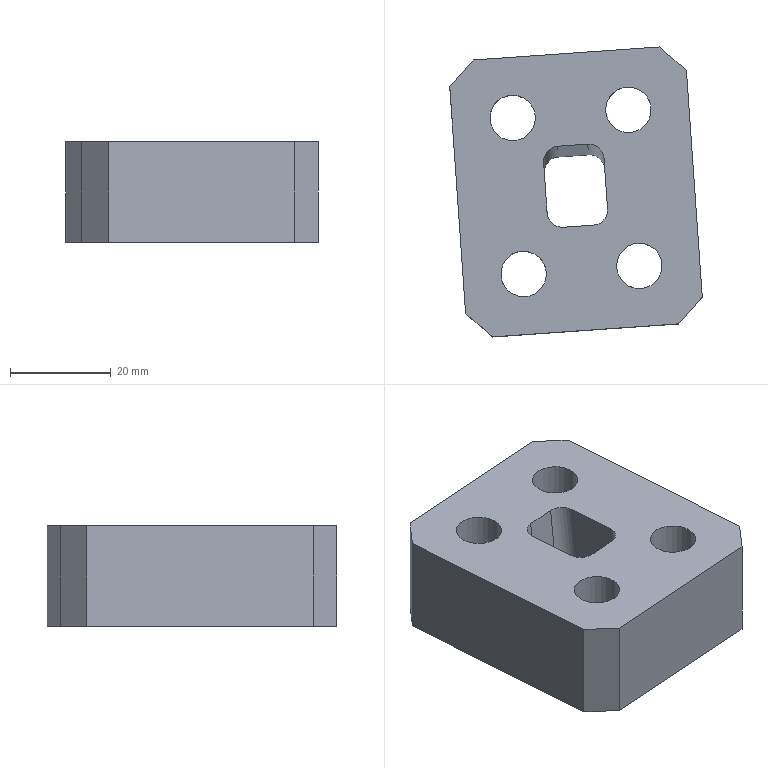Part | STEP file | 车灯-后视镜_id158_x_t | 1 solid | 30 faces | box 50.025 x 57.447 x 20 mm | volume 38834 mm3 | plane 18 | cylinder 12 | commonest cylinder face diameters 6 x4 9 x4 14 x4
STEP:
#1=CARTESIAN_POINT('',(-10.346,-54.305,-160.5));
#2=VERTEX_POINT('',#1);
#3=CARTESIAN_POINT('',(-10.346,-61.305,-160.5));
#4=DIRECTION('',(0.,0.,1.));
#5=DIRECTION('',(0.,1.,0.));
#6=AXIS2_PLACEMENT_3D('',#3,#4,#5);
#7=CIRCLE('',#6,7.);
#8=EDGE_CURVE('',#2,#2,#7,.T.);
#9=ORIENTED_EDGE('',*,*,#8,.T.);
#10=EDGE_LOOP('',(#9));
#11=FACE_BOUND('',#10,.T.);
#12=CARTESIAN_POINT('',(-8.184,-85.229,-160.5));
#13=VERTEX_POINT('',#12);
#14=CARTESIAN_POINT('',(-8.184,-92.229,-160.5));
#15=DIRECTION('',(0.,0.,-1.));
#16=DIRECTION('',(0.,1.,0.));
#17=AXIS2_PLACEMENT_3D('',#14,#15,#16);
#18=CIRCLE('',#17,7.);
#19=EDGE_CURVE('',#13,#13,#18,.T.);
#20=ORIENTED_EDGE('',*,*,#19,.F.);
#21=EDGE_LOOP('',(#20));
#22=FACE_BOUND('',#21,.T.);
#23=CARTESIAN_POINT('',(12.598,-52.7,-160.5));
#24=VERTEX_POINT('',#23);
#25=CARTESIAN_POINT('',(12.598,-59.7,-160.5));
#26=DIRECTION('',(0.,0.,-1.));
#27=DIRECTION('',(0.,1.,0.));
#28=AXIS2_PLACEMENT_3D('',#25,#26,#27);
#29=CIRCLE('',#28,7.);
#30=EDGE_CURVE('',#24,#24,#29,.T.);
#31=ORIENTED_EDGE('',*,*,#30,.F.);
#32=EDGE_LOOP('',(#31));
#33=FACE_BOUND('',#32,.T.);
#34=CARTESIAN_POINT('',(14.76,-83.625,-160.5));
#35=VERTEX_POINT('',#34);
#36=CARTESIAN_POINT('',(14.76,-90.625,-160.5));
#37=DIRECTION('',(0.,0.,1.));
#38=DIRECTION('',(0.,1.,0.));
#39=AXIS2_PLACEMENT_3D('',#36,#37,#38);
#40=CIRCLE('',#39,7.);
#41=EDGE_CURVE('',#35,#35,#40,.T.);
#42=ORIENTED_EDGE('',*,*,#41,.T.);
#43=EDGE_LOOP('',(#42));
#44=FACE_BOUND('',#43,.T.);
#45=CARTESIAN_POINT('',(-18.166,-49.822,-160.5));
#46=VERTEX_POINT('',#45);
#47=CARTESIAN_POINT('',(18.744,-47.241,-160.5));
#48=VERTEX_POINT('',#47);
#49=CARTESIAN_POINT('',(0.8645,-48.491,-160.5));
#50=DIRECTION('',(0.9976,0.06976,0.));
#51=VECTOR('',#50,1.);
#52=LINE('',#49,#51);
#53=EDGE_CURVE('',#46,#48,#52,.T.);
#54=ORIENTED_EDGE('',*,*,#53,.T.);
#55=CARTESIAN_POINT('',(24.08,-51.88,-160.5));
#56=VERTEX_POINT('',#55);
#57=CARTESIAN_POINT('',(18.744,-47.241,-160.5));
#58=DIRECTION('',(-0.7547,0.6561,0.));
#59=VECTOR('',#58,1.);
#60=LINE('',#57,#59);
#61=EDGE_CURVE('',#56,#48,#60,.T.);
#62=ORIENTED_EDGE('',*,*,#61,.F.);
#63=CARTESIAN_POINT('',(27.219,-96.771,-160.5));
#64=VERTEX_POINT('',#63);
#65=CARTESIAN_POINT('',(26.697,-89.301,-160.5));
#66=DIRECTION('',(0.06976,-0.9976,0.));
#67=VECTOR('',#66,1.);
#68=LINE('',#65,#67);
#69=EDGE_CURVE('',#56,#64,#68,.T.);
#70=ORIENTED_EDGE('',*,*,#69,.T.);
#71=CARTESIAN_POINT('',(22.58,-102.107,-160.5));
#72=VERTEX_POINT('',#71);
#73=CARTESIAN_POINT('',(22.58,-102.107,-160.5));
#74=DIRECTION('',(0.6561,0.7547,0.));
#75=VECTOR('',#74,1.);
#76=LINE('',#73,#75);
#77=EDGE_CURVE('',#72,#64,#76,.T.);
#78=ORIENTED_EDGE('',*,*,#77,.F.);
#79=CARTESIAN_POINT('',(-14.33,-104.688,-160.5));
#80=VERTEX_POINT('',#79);
#81=CARTESIAN_POINT('',(4.701,-103.357,-160.5));
#82=DIRECTION('',(-0.9976,-0.06976,0.));
#83=VECTOR('',#82,1.);
#84=LINE('',#81,#83);
#85=EDGE_CURVE('',#72,#80,#84,.T.);
#86=ORIENTED_EDGE('',*,*,#85,.T.);
#87=CARTESIAN_POINT('',(-19.666,-100.049,-160.5));
#88=VERTEX_POINT('',#87);
#89=CARTESIAN_POINT('',(-14.33,-104.688,-160.5));
#90=DIRECTION('',(0.7547,-0.6561,0.));
#91=VECTOR('',#90,1.);
#92=LINE('',#89,#91);
#93=EDGE_CURVE('',#88,#80,#92,.T.);
#94=ORIENTED_EDGE('',*,*,#93,.F.);
#95=CARTESIAN_POINT('',(-22.805,-55.159,-160.5));
#96=VERTEX_POINT('',#95);
#97=CARTESIAN_POINT('',(-20.188,-92.579,-160.5));
#98=DIRECTION('',(-0.06976,0.9976,0.));
#99=VECTOR('',#98,1.);
#100=LINE('',#97,#99);
#101=EDGE_CURVE('',#88,#96,#100,.T.);
#102=ORIENTED_EDGE('',*,*,#101,.T.);
#103=CARTESIAN_POINT('',(-22.805,-55.159,-160.5));
#104=DIRECTION('',(-0.6561,-0.7547,0.));
#105=VECTOR('',#104,1.);
#106=LINE('',#103,#105);
#107=EDGE_CURVE('',#46,#96,#106,.T.);
#108=ORIENTED_EDGE('',*,*,#107,.F.);
#109=EDGE_LOOP('',(#54,#62,#70,#78,#86,#94,#102,#108));
#110=FACE_BOUND('',#109,.T.);
#111=CARTESIAN_POINT('',(-4.069,-72.231,-160.5));
#112=VERTEX_POINT('',#111);
#113=CARTESIAN_POINT('',(-1.286,-69.013,-160.5));
#114=VERTEX_POINT('',#113);
#115=CARTESIAN_POINT('',(-1.076,-72.022,-160.5));
#116=DIRECTION('',(0.,0.,-1.));
#117=DIRECTION('',(-0.06976,0.9976,0.));
#118=AXIS2_PLACEMENT_3D('',#115,#116,#117);
#119=ELLIPSE('',#118,3.017,3.);
#120=EDGE_CURVE('',#112,#114,#119,.T.);
#121=ORIENTED_EDGE('',*,*,#120,.F.);
#122=CARTESIAN_POINT('',(-3.367,-82.262,-160.5));
#123=VERTEX_POINT('',#122);
#124=CARTESIAN_POINT('',(-2.731,-91.358,-160.5));
#125=DIRECTION('',(0.06976,-0.9976,0.));
#126=VECTOR('',#125,1.);
#127=LINE('',#124,#126);
#128=EDGE_CURVE('',#112,#123,#127,.T.);
#129=ORIENTED_EDGE('',*,*,#128,.T.);
#130=CARTESIAN_POINT('',(-0.1641,-85.062,-160.5));
#131=VERTEX_POINT('',#130);
#132=CARTESIAN_POINT('',(-0.3745,-82.053,-160.5));
#133=DIRECTION('',(0.,0.,-1.));
#134=DIRECTION('',(0.06976,-0.9976,0.));
#135=AXIS2_PLACEMENT_3D('',#132,#133,#134);
#136=ELLIPSE('',#135,3.017,3.);
#137=EDGE_CURVE('',#131,#123,#136,.T.);
#138=ORIENTED_EDGE('',*,*,#137,.F.);
#139=CARTESIAN_POINT('',(5.821,-84.643,-160.5));
#140=VERTEX_POINT('',#139);
#141=CARTESIAN_POINT('',(3.404,-84.812,-160.5));
#142=DIRECTION('',(-0.9976,-0.06976,0.));
#143=VECTOR('',#142,1.);
#144=LINE('',#141,#143);
#145=EDGE_CURVE('',#140,#131,#144,.T.);
#146=ORIENTED_EDGE('',*,*,#145,.F.);
#147=CARTESIAN_POINT('',(8.604,-81.425,-160.5));
#148=VERTEX_POINT('',#147);
#149=CARTESIAN_POINT('',(5.611,-81.634,-160.5));
#150=DIRECTION('',(0.,0.,-1.));
#151=DIRECTION('',(-0.06976,0.9976,0.));
#152=AXIS2_PLACEMENT_3D('',#149,#150,#151);
#153=ELLIPSE('',#152,3.017,3.);
#154=EDGE_CURVE('',#148,#140,#153,.T.);
#155=ORIENTED_EDGE('',*,*,#154,.F.);
#156=CARTESIAN_POINT('',(7.902,-71.394,-160.5));
#157=VERTEX_POINT('',#156);
#158=CARTESIAN_POINT('',(9.24,-90.521,-160.5));
#159=DIRECTION('',(0.06976,-0.9976,0.));
#160=VECTOR('',#159,1.);
#161=LINE('',#158,#160);
#162=EDGE_CURVE('',#157,#148,#161,.T.);
#163=ORIENTED_EDGE('',*,*,#162,.F.);
#164=CARTESIAN_POINT('',(4.699,-68.594,-160.5));
#165=VERTEX_POINT('',#164);
#166=CARTESIAN_POINT('',(4.909,-71.603,-160.5));
#167=DIRECTION('',(0.,0.,-1.));
#168=DIRECTION('',(0.06976,-0.9976,0.));
#169=AXIS2_PLACEMENT_3D('',#166,#167,#168);
#170=ELLIPSE('',#169,3.017,3.);
#171=EDGE_CURVE('',#165,#157,#170,.T.);
#172=ORIENTED_EDGE('',*,*,#171,.F.);
#173=CARTESIAN_POINT('',(2.282,-68.763,-160.5));
#174=DIRECTION('',(0.9976,0.06976,0.));
#175=VECTOR('',#174,1.);
#176=LINE('',#173,#175);
#177=EDGE_CURVE('',#114,#165,#176,.T.);
#178=ORIENTED_EDGE('',*,*,#177,.F.);
#179=EDGE_LOOP('',(#121,#129,#138,#146,#155,#163,#172,#178));
#180=FACE_BOUND('',#179,.T.);
#181=CARTESIAN_POINT('',(3.83,-90.9,-160.5));
#182=DIRECTION('',(0.,0.,-1.));
#183=DIRECTION('',(-0.06976,0.9976,0.));
#184=AXIS2_PLACEMENT_3D('',#181,#182,#183);
#185=PLANE('',#184);
#186=ADVANCED_FACE('',(#11,#22,#33,#44,#110,#180),#185,.T.);
#187=CARTESIAN_POINT('',(-10.346,-65.805,-140.5));
#188=VERTEX_POINT('',#187);
#189=CARTESIAN_POINT('',(-10.346,-61.305,-140.5));
#190=DIRECTION('',(0.,0.,-1.));
#191=DIRECTION('',(0.,-1.,0.));
#192=AXIS2_PLACEMENT_3D('',#189,#190,#191);
#193=CIRCLE('',#192,4.5);
#194=EDGE_CURVE('',#188,#188,#193,.T.);
#195=ORIENTED_EDGE('',*,*,#194,.T.);
#196=EDGE_LOOP('',(#195));
#197=FACE_BOUND('',#196,.T.);
#198=CARTESIAN_POINT('',(-8.184,-96.729,-140.5));
#199=VERTEX_POINT('',#198);
#200=CARTESIAN_POINT('',(-8.184,-92.229,-140.5));
#201=DIRECTION('',(0.,0.,1.));
#202=DIRECTION('',(0.,-1.,0.));
#203=AXIS2_PLACEMENT_3D('',#200,#201,#202);
#204=CIRCLE('',#203,4.5);
#205=EDGE_CURVE('',#199,#199,#204,.T.);
#206=ORIENTED_EDGE('',*,*,#205,.F.);
#207=EDGE_LOOP('',(#206));
#208=FACE_BOUND('',#207,.T.);
#209=CARTESIAN_POINT('',(12.598,-64.2,-140.5));
#210=VERTEX_POINT('',#209);
#211=CARTESIAN_POINT('',(12.598,-59.7,-140.5));
#212=DIRECTION('',(0.,0.,1.));
#213=DIRECTION('',(0.,-1.,0.));
#214=AXIS2_PLACEMENT_3D('',#211,#212,#213);
#215=CIRCLE('',#214,4.5);
#216=EDGE_CURVE('',#210,#210,#215,.T.);
#217=ORIENTED_EDGE('',*,*,#216,.F.);
#218=EDGE_LOOP('',(#217));
#219=FACE_BOUND('',#218,.T.);
#220=CARTESIAN_POINT('',(14.76,-95.125,-140.5));
#221=VERTEX_POINT('',#220);
#222=CARTESIAN_POINT('',(14.76,-90.625,-140.5));
#223=DIRECTION('',(0.,0.,-1.));
#224=DIRECTION('',(0.,-1.,0.));
#225=AXIS2_PLACEMENT_3D('',#222,#223,#224);
#226=CIRCLE('',#225,4.5);
#227=EDGE_CURVE('',#221,#221,#226,.T.);
#228=ORIENTED_EDGE('',*,*,#227,.T.);
#229=EDGE_LOOP('',(#228));
#230=FACE_BOUND('',#229,.T.);
#231=CARTESIAN_POINT('',(-22.805,-55.159,-140.5));
#232=VERTEX_POINT('',#231);
#233=CARTESIAN_POINT('',(-19.666,-100.049,-140.5));
#234=VERTEX_POINT('',#233);
#235=CARTESIAN_POINT('',(-20.188,-92.579,-140.5));
#236=DIRECTION('',(0.06976,-0.9976,0.));
#237=VECTOR('',#236,1.);
#238=LINE('',#235,#237);
#239=EDGE_CURVE('',#232,#234,#238,.T.);
#240=ORIENTED_EDGE('',*,*,#239,.T.);
#241=CARTESIAN_POINT('',(-14.33,-104.688,-140.5));
#242=VERTEX_POINT('',#241);
#243=CARTESIAN_POINT('',(-14.33,-104.688,-140.5));
#244=DIRECTION('',(-0.7547,0.6561,0.));
#245=VECTOR('',#244,1.);
#246=LINE('',#243,#245);
#247=EDGE_CURVE('',#242,#234,#246,.T.);
#248=ORIENTED_EDGE('',*,*,#247,.F.);
#249=CARTESIAN_POINT('',(22.58,-102.107,-140.5));
#250=VERTEX_POINT('',#249);
#251=CARTESIAN_POINT('',(4.701,-103.357,-140.5));
#252=DIRECTION('',(0.9976,0.06976,0.));
#253=VECTOR('',#252,1.);
#254=LINE('',#251,#253);
#255=EDGE_CURVE('',#242,#250,#254,.T.);
#256=ORIENTED_EDGE('',*,*,#255,.T.);
#257=CARTESIAN_POINT('',(27.219,-96.771,-140.5));
#258=VERTEX_POINT('',#257);
#259=CARTESIAN_POINT('',(22.58,-102.107,-140.5));
#260=DIRECTION('',(-0.6561,-0.7547,0.));
#261=VECTOR('',#260,1.);
#262=LINE('',#259,#261);
#263=EDGE_CURVE('',#258,#250,#262,.T.);
#264=ORIENTED_EDGE('',*,*,#263,.F.);
#265=CARTESIAN_POINT('',(24.08,-51.88,-140.5));
#266=VERTEX_POINT('',#265);
#267=CARTESIAN_POINT('',(26.697,-89.301,-140.5));
#268=DIRECTION('',(-0.06976,0.9976,0.));
#269=VECTOR('',#268,1.);
#270=LINE('',#267,#269);
#271=EDGE_CURVE('',#258,#266,#270,.T.);
#272=ORIENTED_EDGE('',*,*,#271,.T.);
#273=CARTESIAN_POINT('',(18.744,-47.241,-140.5));
#274=VERTEX_POINT('',#273);
#275=CARTESIAN_POINT('',(18.744,-47.241,-140.5));
#276=DIRECTION('',(0.7547,-0.6561,0.));
#277=VECTOR('',#276,1.);
#278=LINE('',#275,#277);
#279=EDGE_CURVE('',#274,#266,#278,.T.);
#280=ORIENTED_EDGE('',*,*,#279,.F.);
#281=CARTESIAN_POINT('',(-18.166,-49.822,-140.5));
#282=VERTEX_POINT('',#281);
#283=CARTESIAN_POINT('',(0.8645,-48.491,-140.5));
#284=DIRECTION('',(-0.9976,-0.06976,0.));
#285=VECTOR('',#284,1.);
#286=LINE('',#283,#285);
#287=EDGE_CURVE('',#274,#282,#286,.T.);
#288=ORIENTED_EDGE('',*,*,#287,.T.);
#289=CARTESIAN_POINT('',(-22.805,-55.159,-140.5));
#290=DIRECTION('',(0.6561,0.7547,0.));
#291=VECTOR('',#290,1.);
#292=LINE('',#289,#291);
#293=EDGE_CURVE('',#232,#282,#292,.T.);
#294=ORIENTED_EDGE('',*,*,#293,.F.);
#295=EDGE_LOOP('',(#240,#248,#256,#264,#272,#280,#288,#294));
#296=FACE_BOUND('',#295,.T.);
#297=CARTESIAN_POINT('',(-3.514,-80.165,-140.5));
#298=VERTEX_POINT('',#297);
#299=CARTESIAN_POINT('',(-0.3107,-82.965,-140.5));
#300=VERTEX_POINT('',#299);
#301=CARTESIAN_POINT('',(-0.5212,-79.956,-140.5));
#302=DIRECTION('',(0.,0.,1.));
#303=DIRECTION('',(0.06976,-0.9976,0.));
#304=AXIS2_PLACEMENT_3D('',#301,#302,#303);
#305=ELLIPSE('',#304,3.017,3.);
#306=EDGE_CURVE('',#298,#300,#305,.T.);
#307=ORIENTED_EDGE('',*,*,#306,.F.);
#308=CARTESIAN_POINT('',(-4.215,-70.134,-140.5));
#309=VERTEX_POINT('',#308);
#310=CARTESIAN_POINT('',(-2.731,-91.358,-140.5));
#311=DIRECTION('',(-0.06976,0.9976,0.));
#312=VECTOR('',#311,1.);
#313=LINE('',#310,#312);
#314=EDGE_CURVE('',#298,#309,#313,.T.);
#315=ORIENTED_EDGE('',*,*,#314,.T.);
#316=CARTESIAN_POINT('',(-1.433,-66.916,-140.5));
#317=VERTEX_POINT('',#316);
#318=CARTESIAN_POINT('',(-1.223,-69.925,-140.5));
#319=DIRECTION('',(0.,0.,1.));
#320=DIRECTION('',(-0.06976,0.9976,0.));
#321=AXIS2_PLACEMENT_3D('',#318,#319,#320);
#322=ELLIPSE('',#321,3.017,3.);
#323=EDGE_CURVE('',#317,#309,#322,.T.);
#324=ORIENTED_EDGE('',*,*,#323,.F.);
#325=CARTESIAN_POINT('',(4.552,-66.497,-140.5));
#326=VERTEX_POINT('',#325);
#327=CARTESIAN_POINT('',(2.135,-66.666,-140.5));
#328=DIRECTION('',(-0.9976,-0.06976,0.));
#329=VECTOR('',#328,1.);
#330=LINE('',#327,#329);
#331=EDGE_CURVE('',#326,#317,#330,.T.);
#332=ORIENTED_EDGE('',*,*,#331,.F.);
#333=CARTESIAN_POINT('',(7.756,-69.297,-140.5));
#334=VERTEX_POINT('',#333);
#335=CARTESIAN_POINT('',(4.763,-69.506,-140.5));
#336=DIRECTION('',(0.,0.,1.));
#337=DIRECTION('',(0.06976,-0.9976,0.));
#338=AXIS2_PLACEMENT_3D('',#335,#336,#337);
#339=ELLIPSE('',#338,3.017,3.);
#340=EDGE_CURVE('',#334,#326,#339,.T.);
#341=ORIENTED_EDGE('',*,*,#340,.F.);
#342=CARTESIAN_POINT('',(8.457,-79.328,-140.5));
#343=VERTEX_POINT('',#342);
#344=CARTESIAN_POINT('',(9.24,-90.521,-140.5));
#345=DIRECTION('',(-0.06976,0.9976,0.));
#346=VECTOR('',#345,1.);
#347=LINE('',#344,#346);
#348=EDGE_CURVE('',#343,#334,#347,.T.);
#349=ORIENTED_EDGE('',*,*,#348,.F.);
#350=CARTESIAN_POINT('',(5.675,-82.546,-140.5));
#351=VERTEX_POINT('',#350);
#352=CARTESIAN_POINT('',(5.464,-79.537,-140.5));
#353=DIRECTION('',(0.,0.,1.));
#354=DIRECTION('',(-0.06976,0.9976,0.));
#355=AXIS2_PLACEMENT_3D('',#352,#353,#354);
#356=ELLIPSE('',#355,3.017,3.);
#357=EDGE_CURVE('',#351,#343,#356,.T.);
#358=ORIENTED_EDGE('',*,*,#357,.F.);
#359=CARTESIAN_POINT('',(3.258,-82.715,-140.5));
#360=DIRECTION('',(0.9976,0.06976,0.));
#361=VECTOR('',#360,1.);
#362=LINE('',#359,#361);
#363=EDGE_CURVE('',#300,#351,#362,.T.);
#364=ORIENTED_EDGE('',*,*,#363,.F.);
#365=EDGE_LOOP('',(#307,#315,#324,#332,#341,#349,#358,#364));
#366=FACE_BOUND('',#365,.T.);
#367=CARTESIAN_POINT('',(3.83,-90.9,-140.5));
#368=DIRECTION('',(0.,0.,1.));
#369=DIRECTION('',(0.06976,-0.9976,0.));
#370=AXIS2_PLACEMENT_3D('',#367,#368,#369);
#371=PLANE('',#370);
#372=ADVANCED_FACE('',(#197,#208,#219,#230,#296,#366),#371,.T.);
#373=ORIENTED_EDGE('',*,*,#271,.F.);
#374=CARTESIAN_POINT('',(27.219,-96.771,-144.5));
#375=DIRECTION('',(0.,0.,1.));
#376=VECTOR('',#375,1.);
#377=LINE('',#374,#376);
#378=EDGE_CURVE('',#64,#258,#377,.T.);
#379=ORIENTED_EDGE('',*,*,#378,.F.);
#380=ORIENTED_EDGE('',*,*,#69,.F.);
#381=CARTESIAN_POINT('',(24.08,-51.88,-138.5));
#382=DIRECTION('',(0.,0.,-1.));
#383=VECTOR('',#382,1.);
#384=LINE('',#381,#383);
#385=EDGE_CURVE('',#266,#56,#384,.T.);
#386=ORIENTED_EDGE('',*,*,#385,.F.);
#387=EDGE_LOOP('',(#373,#379,#380,#386));
#388=FACE_OUTER_BOUND('',#387,.T.);
#389=CARTESIAN_POINT('',(26.697,-89.301,-138.5));
#390=DIRECTION('',(0.9976,0.06976,0.));
#391=DIRECTION('',(0.,0.,1.));
#392=AXIS2_PLACEMENT_3D('',#389,#390,#391);
#393=PLANE('',#392);
#394=ADVANCED_FACE('',(#388),#393,.T.);
#395=ORIENTED_EDGE('',*,*,#101,.F.);
#396=CARTESIAN_POINT('',(-19.666,-100.049,-144.5));
#397=DIRECTION('',(0.,0.,-1.));
#398=VECTOR('',#397,1.);
#399=LINE('',#396,#398);
#400=EDGE_CURVE('',#234,#88,#399,.T.);
#401=ORIENTED_EDGE('',*,*,#400,.F.);
#402=ORIENTED_EDGE('',*,*,#239,.F.);
#403=CARTESIAN_POINT('',(-22.805,-55.159,-138.5));
#404=DIRECTION('',(0.,0.,1.));
#405=VECTOR('',#404,1.);
#406=LINE('',#403,#405);
#407=EDGE_CURVE('',#96,#232,#406,.T.);
#408=ORIENTED_EDGE('',*,*,#407,.F.);
#409=EDGE_LOOP('',(#395,#401,#402,#408));
#410=FACE_OUTER_BOUND('',#409,.T.);
#411=CARTESIAN_POINT('',(-20.188,-92.579,-138.5));
#412=DIRECTION('',(-0.9976,-0.06976,0.));
#413=DIRECTION('',(0.,0.,-1.));
#414=AXIS2_PLACEMENT_3D('',#411,#412,#413);
#415=PLANE('',#414);
#416=ADVANCED_FACE('',(#410),#415,.T.);
#417=ORIENTED_EDGE('',*,*,#287,.F.);
#418=CARTESIAN_POINT('',(18.744,-47.241,-138.5));
#419=DIRECTION('',(0.,0.,1.));
#420=VECTOR('',#419,1.);
#421=LINE('',#418,#420);
#422=EDGE_CURVE('',#48,#274,#421,.T.);
#423=ORIENTED_EDGE('',*,*,#422,.F.);
#424=ORIENTED_EDGE('',*,*,#53,.F.);
#425=CARTESIAN_POINT('',(-18.166,-49.822,-138.5));
#426=DIRECTION('',(0.,0.,-1.));
#427=VECTOR('',#426,1.);
#428=LINE('',#425,#427);
#429=EDGE_CURVE('',#282,#46,#428,.T.);
#430=ORIENTED_EDGE('',*,*,#429,.F.);
#431=EDGE_LOOP('',(#417,#423,#424,#430));
#432=FACE_OUTER_BOUND('',#431,.T.);
#433=CARTESIAN_POINT('',(0.8645,-48.491,-138.5));
#434=DIRECTION('',(-0.06976,0.9976,0.));
#435=DIRECTION('',(0.,0.,1.));
#436=AXIS2_PLACEMENT_3D('',#433,#434,#435);
#437=PLANE('',#436);
#438=ADVANCED_FACE('',(#432),#437,.T.);
#439=CARTESIAN_POINT('',(-10.385,-56.805,-152.));
#440=VERTEX_POINT('',#439);
#441=CARTESIAN_POINT('',(-10.346,-61.305,-152.));
#442=DIRECTION('',(0.,0.,-1.));
#443=DIRECTION('',(-0.008727,1.,0.));
#444=AXIS2_PLACEMENT_3D('',#441,#442,#443);
#445=CIRCLE('',#444,4.5);
#446=EDGE_CURVE('',#440,#440,#445,.T.);
#447=ORIENTED_EDGE('',*,*,#446,.T.);
#448=EDGE_LOOP('',(#447));
#449=FACE_BOUND('',#448,.T.);
#450=ORIENTED_EDGE('',*,*,#194,.F.);
#451=EDGE_LOOP('',(#450));
#452=FACE_BOUND('',#451,.T.);
#453=CARTESIAN_POINT('',(-10.346,-61.305,-140.5));
#454=DIRECTION('',(0.,0.,-1.));
#455=DIRECTION('',(0.06976,-0.9976,0.));
#456=AXIS2_PLACEMENT_3D('',#453,#454,#455);
#457=CYLINDRICAL_SURFACE('',#456,4.5);
#458=ADVANCED_FACE('',(#449,#452),#457,.F.);
#459=ORIENTED_EDGE('',*,*,#446,.F.);
#460=EDGE_LOOP('',(#459));
#461=FACE_BOUND('',#460,.T.);
#462=CARTESIAN_POINT('',(-10.407,-54.305,-152.));
#463=VERTEX_POINT('',#462);
#464=CARTESIAN_POINT('',(-10.346,-61.305,-152.));
#465=DIRECTION('',(0.,0.,-1.));
#466=DIRECTION('',(-0.008727,1.,0.));
#467=AXIS2_PLACEMENT_3D('',#464,#465,#466);
#468=CIRCLE('',#467,7.);
#469=EDGE_CURVE('',#463,#463,#468,.T.);
#470=ORIENTED_EDGE('',*,*,#469,.T.);
#471=EDGE_LOOP('',(#470));
#472=FACE_BOUND('',#471,.T.);
#473=CARTESIAN_POINT('',(-10.346,-61.305,-152.));
#474=DIRECTION('',(0.,0.,1.));
#475=DIRECTION('',(-0.06976,0.9976,0.));
#476=AXIS2_PLACEMENT_3D('',#473,#474,#475);
#477=PLANE('',#476);
#478=ADVANCED_FACE('',(#461,#472),#477,.F.);
#479=ORIENTED_EDGE('',*,*,#469,.F.);
#480=EDGE_LOOP('',(#479));
#481=FACE_BOUND('',#480,.T.);
#482=ORIENTED_EDGE('',*,*,#8,.F.);
#483=EDGE_LOOP('',(#482));
#484=FACE_BOUND('',#483,.T.);
#485=CARTESIAN_POINT('',(-10.346,-61.305,-150.5));
#486=DIRECTION('',(0.,0.,1.));
#487=DIRECTION('',(-0.06976,0.9976,0.));
#488=AXIS2_PLACEMENT_3D('',#485,#486,#487);
#489=CYLINDRICAL_SURFACE('',#488,7.);
#490=ADVANCED_FACE('',(#481,#484),#489,.F.);
#491=CARTESIAN_POINT('',(-8.223,-87.729,-152.));
#492=VERTEX_POINT('',#491);
#493=CARTESIAN_POINT('',(-8.184,-92.229,-152.));
#494=DIRECTION('',(0.,0.,1.));
#495=DIRECTION('',(-0.008727,1.,0.));
#496=AXIS2_PLACEMENT_3D('',#493,#494,#495);
#497=CIRCLE('',#496,4.5);
#498=EDGE_CURVE('',#492,#492,#497,.T.);
#499=ORIENTED_EDGE('',*,*,#498,.F.);
#500=EDGE_LOOP('',(#499));
#501=FACE_BOUND('',#500,.T.);
#502=ORIENTED_EDGE('',*,*,#205,.T.);
#503=EDGE_LOOP('',(#502));
#504=FACE_BOUND('',#503,.T.);
#505=CARTESIAN_POINT('',(-8.184,-92.229,-140.5));
#506=DIRECTION('',(0.,0.,-1.));
#507=DIRECTION('',(-0.06976,0.9976,0.));
#508=AXIS2_PLACEMENT_3D('',#505,#506,#507);
#509=CYLINDRICAL_SURFACE('',#508,4.5);
#510=ADVANCED_FACE('',(#501,#504),#509,.F.);
#511=ORIENTED_EDGE('',*,*,#498,.T.);
#512=EDGE_LOOP('',(#511));
#513=FACE_BOUND('',#512,.T.);
#514=CARTESIAN_POINT('',(-8.245,-85.229,-152.));
#515=VERTEX_POINT('',#514);
#516=CARTESIAN_POINT('',(-8.184,-92.229,-152.));
#517=DIRECTION('',(0.,0.,1.));
#518=DIRECTION('',(-0.008727,1.,0.));
#519=AXIS2_PLACEMENT_3D('',#516,#517,#518);
#520=CIRCLE('',#519,7.);
#521=EDGE_CURVE('',#515,#515,#520,.T.);
#522=ORIENTED_EDGE('',*,*,#521,.F.);
#523=EDGE_LOOP('',(#522));
#524=FACE_BOUND('',#523,.T.);
#525=CARTESIAN_POINT('',(-8.184,-92.229,-152.));
#526=DIRECTION('',(0.,0.,1.));
#527=DIRECTION('',(0.06976,-0.9976,0.));
#528=AXIS2_PLACEMENT_3D('',#525,#526,#527);
#529=PLANE('',#528);
#530=ADVANCED_FACE('',(#513,#524),#529,.F.);
#531=ORIENTED_EDGE('',*,*,#521,.T.);
#532=EDGE_LOOP('',(#531));
#533=FACE_BOUND('',#532,.T.);
#534=ORIENTED_EDGE('',*,*,#19,.T.);
#535=EDGE_LOOP('',(#534));
#536=FACE_BOUND('',#535,.T.);
#537=CARTESIAN_POINT('',(-8.184,-92.229,-150.5));
#538=DIRECTION('',(0.,0.,1.));
#539=DIRECTION('',(0.06976,-0.9976,0.));
#540=AXIS2_PLACEMENT_3D('',#537,#538,#539);
#541=CYLINDRICAL_SURFACE('',#540,7.);
#542=ADVANCED_FACE('',(#533,#536),#541,.F.);
#543=CARTESIAN_POINT('',(12.559,-55.2,-152.));
#544=VERTEX_POINT('',#543);
#545=CARTESIAN_POINT('',(12.598,-59.7,-152.));
#546=DIRECTION('',(0.,0.,1.));
#547=DIRECTION('',(-0.008727,1.,0.));
#548=AXIS2_PLACEMENT_3D('',#545,#546,#547);
#549=CIRCLE('',#548,4.5);
#550=EDGE_CURVE('',#544,#544,#549,.T.);
#551=ORIENTED_EDGE('',*,*,#550,.F.);
#552=EDGE_LOOP('',(#551));
#553=FACE_BOUND('',#552,.T.);
#554=ORIENTED_EDGE('',*,*,#216,.T.);
#555=EDGE_LOOP('',(#554));
#556=FACE_BOUND('',#555,.T.);
#557=CARTESIAN_POINT('',(12.598,-59.7,-140.5));
#558=DIRECTION('',(0.,0.,-1.));
#559=DIRECTION('',(0.06976,-0.9976,0.));
#560=AXIS2_PLACEMENT_3D('',#557,#558,#559);
#561=CYLINDRICAL_SURFACE('',#560,4.5);
#562=ADVANCED_FACE('',(#553,#556),#561,.F.);
#563=ORIENTED_EDGE('',*,*,#550,.T.);
#564=EDGE_LOOP('',(#563));
#565=FACE_BOUND('',#564,.T.);
#566=CARTESIAN_POINT('',(12.537,-52.7,-152.));
#567=VERTEX_POINT('',#566);
#568=CARTESIAN_POINT('',(12.598,-59.7,-152.));
#569=DIRECTION('',(0.,0.,1.));
#570=DIRECTION('',(-0.008727,1.,0.));
#571=AXIS2_PLACEMENT_3D('',#568,#569,#570);
#572=CIRCLE('',#571,7.);
#573=EDGE_CURVE('',#567,#567,#572,.T.);
#574=ORIENTED_EDGE('',*,*,#573,.F.);
#575=EDGE_LOOP('',(#574));
#576=FACE_BOUND('',#575,.T.);
#577=CARTESIAN_POINT('',(12.598,-59.7,-152.));
#578=DIRECTION('',(0.,0.,1.));
#579=DIRECTION('',(-0.06976,0.9976,0.));
#580=AXIS2_PLACEMENT_3D('',#577,#578,#579);
#581=PLANE('',#580);
#582=ADVANCED_FACE('',(#565,#576),#581,.F.);
#583=ORIENTED_EDGE('',*,*,#573,.T.);
#584=EDGE_LOOP('',(#583));
#585=FACE_BOUND('',#584,.T.);
#586=ORIENTED_EDGE('',*,*,#30,.T.);
#587=EDGE_LOOP('',(#586));
#588=FACE_BOUND('',#587,.T.);
#589=CARTESIAN_POINT('',(12.598,-59.7,-150.5));
#590=DIRECTION('',(0.,0.,1.));
#591=DIRECTION('',(-0.06976,0.9976,0.));
#592=AXIS2_PLACEMENT_3D('',#589,#590,#591);
#593=CYLINDRICAL_SURFACE('',#592,7.);
#594=ADVANCED_FACE('',(#585,#588),#593,.F.);
#595=CARTESIAN_POINT('',(14.721,-86.125,-152.));
#596=VERTEX_POINT('',#595);
#597=CARTESIAN_POINT('',(14.76,-90.625,-152.));
#598=DIRECTION('',(0.,0.,-1.));
#599=DIRECTION('',(-0.008727,1.,0.));
#600=AXIS2_PLACEMENT_3D('',#597,#598,#599);
#601=CIRCLE('',#600,4.5);
#602=EDGE_CURVE('',#596,#596,#601,.T.);
#603=ORIENTED_EDGE('',*,*,#602,.T.);
#604=EDGE_LOOP('',(#603));
#605=FACE_BOUND('',#604,.T.);
#606=ORIENTED_EDGE('',*,*,#227,.F.);
#607=EDGE_LOOP('',(#606));
#608=FACE_BOUND('',#607,.T.);
#609=CARTESIAN_POINT('',(14.76,-90.625,-140.5));
#610=DIRECTION('',(0.,0.,-1.));
#611=DIRECTION('',(-0.06976,0.9976,0.));
#612=AXIS2_PLACEMENT_3D('',#609,#610,#611);
#613=CYLINDRICAL_SURFACE('',#612,4.5);
#614=ADVANCED_FACE('',(#605,#608),#613,.F.);
#615=ORIENTED_EDGE('',*,*,#602,.F.);
#616=EDGE_LOOP('',(#615));
#617=FACE_BOUND('',#616,.T.);
#618=CARTESIAN_POINT('',(14.699,-83.625,-152.));
#619=VERTEX_POINT('',#618);
#620=CARTESIAN_POINT('',(14.76,-90.625,-152.));
#621=DIRECTION('',(0.,0.,-1.));
#622=DIRECTION('',(-0.008727,1.,0.));
#623=AXIS2_PLACEMENT_3D('',#620,#621,#622);
#624=CIRCLE('',#623,7.);
#625=EDGE_CURVE('',#619,#619,#624,.T.);
#626=ORIENTED_EDGE('',*,*,#625,.T.);
#627=EDGE_LOOP('',(#626));
#628=FACE_BOUND('',#627,.T.);
#629=CARTESIAN_POINT('',(14.76,-90.625,-152.));
#630=DIRECTION('',(0.,0.,1.));
#631=DIRECTION('',(0.06976,-0.9976,0.));
#632=AXIS2_PLACEMENT_3D('',#629,#630,#631);
#633=PLANE('',#632);
#634=ADVANCED_FACE('',(#617,#628),#633,.F.);
#635=ORIENTED_EDGE('',*,*,#625,.F.);
#636=EDGE_LOOP('',(#635));
#637=FACE_BOUND('',#636,.T.);
#638=ORIENTED_EDGE('',*,*,#41,.F.);
#639=EDGE_LOOP('',(#638));
#640=FACE_BOUND('',#639,.T.);
#641=CARTESIAN_POINT('',(14.76,-90.625,-150.5));
#642=DIRECTION('',(0.,0.,1.));
#643=DIRECTION('',(0.06976,-0.9976,0.));
#644=AXIS2_PLACEMENT_3D('',#641,#642,#643);
#645=CYLINDRICAL_SURFACE('',#644,7.);
#646=ADVANCED_FACE('',(#637,#640),#645,.F.);
#647=ORIENTED_EDGE('',*,*,#255,.F.);
#648=CARTESIAN_POINT('',(-14.33,-104.688,-144.5));
#649=DIRECTION('',(0.,0.,1.));
#650=VECTOR('',#649,1.);
#651=LINE('',#648,#650);
#652=EDGE_CURVE('',#80,#242,#651,.T.);
#653=ORIENTED_EDGE('',*,*,#652,.F.);
#654=ORIENTED_EDGE('',*,*,#85,.F.);
#655=CARTESIAN_POINT('',(22.58,-102.107,-144.5));
#656=DIRECTION('',(0.,0.,-1.));
#657=VECTOR('',#656,1.);
#658=LINE('',#655,#657);
#659=EDGE_CURVE('',#250,#72,#658,.T.);
#660=ORIENTED_EDGE('',*,*,#659,.F.);
#661=EDGE_LOOP('',(#647,#653,#654,#660));
#662=FACE_OUTER_BOUND('',#661,.T.);
#663=CARTESIAN_POINT('',(4.701,-103.357,-144.5));
#664=DIRECTION('',(-0.06976,0.9976,0.));
#665=DIRECTION('',(0.,0.,-1.));
#666=AXIS2_PLACEMENT_3D('',#663,#664,#665);
#667=PLANE('',#666);
#668=ADVANCED_FACE('',(#662),#667,.F.);
#669=ORIENTED_EDGE('',*,*,#263,.T.);
#670=ORIENTED_EDGE('',*,*,#659,.T.);
#671=ORIENTED_EDGE('',*,*,#77,.T.);
#672=ORIENTED_EDGE('',*,*,#378,.T.);
#673=EDGE_LOOP('',(#669,#670,#671,#672));
#674=FACE_OUTER_BOUND('',#673,.T.);
#675=CARTESIAN_POINT('',(22.58,-102.107,-144.5));
#676=DIRECTION('',(0.7547,-0.6561,0.));
#677=DIRECTION('',(0.6561,0.7547,0.));
#678=AXIS2_PLACEMENT_3D('',#675,#676,#677);
#679=PLANE('',#678);
#680=ADVANCED_FACE('',(#674),#679,.T.);
#681=ORIENTED_EDGE('',*,*,#93,.T.);
#682=ORIENTED_EDGE('',*,*,#652,.T.);
#683=ORIENTED_EDGE('',*,*,#247,.T.);
#684=ORIENTED_EDGE('',*,*,#400,.T.);
#685=EDGE_LOOP('',(#681,#682,#683,#684));
#686=FACE_OUTER_BOUND('',#685,.T.);
#687=CARTESIAN_POINT('',(-14.33,-104.688,-144.5));
#688=DIRECTION('',(-0.6561,-0.7547,0.));
#689=DIRECTION('',(0.7547,-0.6561,0.));
#690=AXIS2_PLACEMENT_3D('',#687,#688,#689);
#691=PLANE('',#690);
#692=ADVANCED_FACE('',(#686),#691,.T.);
#693=ORIENTED_EDGE('',*,*,#107,.T.);
#694=ORIENTED_EDGE('',*,*,#407,.T.);
#695=ORIENTED_EDGE('',*,*,#293,.T.);
#696=ORIENTED_EDGE('',*,*,#429,.T.);
#697=EDGE_LOOP('',(#693,#694,#695,#696));
#698=FACE_OUTER_BOUND('',#697,.T.);
#699=CARTESIAN_POINT('',(-22.805,-55.159,-138.5));
#700=DIRECTION('',(0.7547,-0.6561,0.));
#701=DIRECTION('',(0.6561,0.7547,0.));
#702=AXIS2_PLACEMENT_3D('',#699,#700,#701);
#703=PLANE('',#702);
#704=ADVANCED_FACE('',(#698),#703,.F.);
#705=ORIENTED_EDGE('',*,*,#61,.T.);
#706=ORIENTED_EDGE('',*,*,#422,.T.);
#707=ORIENTED_EDGE('',*,*,#279,.T.);
#708=ORIENTED_EDGE('',*,*,#385,.T.);
#709=EDGE_LOOP('',(#705,#706,#707,#708));
#710=FACE_OUTER_BOUND('',#709,.T.);
#711=CARTESIAN_POINT('',(18.744,-47.241,-138.5));
#712=DIRECTION('',(-0.6561,-0.7547,0.));
#713=DIRECTION('',(0.7547,-0.6561,0.));
#714=AXIS2_PLACEMENT_3D('',#711,#712,#713);
#715=PLANE('',#714);
#716=ADVANCED_FACE('',(#710),#715,.F.);
#717=CARTESIAN_POINT('',(-5.376,-53.535,17.813));
#718=DIRECTION('',(0.007292,-0.1043,-0.9945));
#719=VECTOR('',#718,1.);
#720=LINE('',#717,#719);
#721=EDGE_CURVE('',#309,#112,#720,.T.);
#722=ORIENTED_EDGE('',*,*,#721,.F.);
#723=ORIENTED_EDGE('',*,*,#314,.F.);
#724=CARTESIAN_POINT('',(-4.861,-60.906,43.186));
#725=DIRECTION('',(-0.007292,0.1043,0.9945));
#726=VECTOR('',#725,1.);
#727=LINE('',#724,#726);
#728=EDGE_CURVE('',#123,#298,#727,.T.);
#729=ORIENTED_EDGE('',*,*,#728,.F.);
#730=ORIENTED_EDGE('',*,*,#128,.F.);
#731=EDGE_LOOP('',(#722,#723,#729,#730));
#732=FACE_OUTER_BOUND('',#731,.T.);
#733=CARTESIAN_POINT('',(-4.072,-72.183,49.203));
#734=DIRECTION('',(0.9976,0.06976,0.));
#735=DIRECTION('',(-0.06976,0.9976,0.));
#736=AXIS2_PLACEMENT_3D('',#733,#734,#735);
#737=PLANE('',#736);
#738=ADVANCED_FACE('',(#732),#737,.T.);
#739=ORIENTED_EDGE('',*,*,#137,.T.);
#740=ORIENTED_EDGE('',*,*,#728,.T.);
#741=ORIENTED_EDGE('',*,*,#306,.T.);
#742=CARTESIAN_POINT('',(-1.469,-66.399,17.5));
#743=DIRECTION('',(0.007292,-0.1043,-0.9945));
#744=VECTOR('',#743,1.);
#745=LINE('',#742,#744);
#746=EDGE_CURVE('',#300,#131,#745,.T.);
#747=ORIENTED_EDGE('',*,*,#746,.T.);
#748=EDGE_LOOP('',(#739,#740,#741,#747));
#749=FACE_OUTER_BOUND('',#748,.T.);
#750=CARTESIAN_POINT('',(-1.903,-60.196,47.963));
#751=DIRECTION('',(0.007292,-0.1043,-0.9945));
#752=DIRECTION('',(0.,0.9945,-0.1043));
#753=AXIS2_PLACEMENT_3D('',#750,#751,#752);
#754=CYLINDRICAL_SURFACE('',#753,3.);
#755=ADVANCED_FACE('',(#749),#754,.F.);
#756=ORIENTED_EDGE('',*,*,#120,.T.);
#757=CARTESIAN_POINT('',(-2.782,-47.624,43.5));
#758=DIRECTION('',(-0.007292,0.1043,0.9945));
#759=VECTOR('',#758,1.);
#760=LINE('',#757,#759);
#761=EDGE_CURVE('',#114,#317,#760,.T.);
#762=ORIENTED_EDGE('',*,*,#761,.T.);
#763=ORIENTED_EDGE('',*,*,#323,.T.);
#764=ORIENTED_EDGE('',*,*,#721,.T.);
#765=EDGE_LOOP('',(#756,#762,#763,#764));
#766=FACE_OUTER_BOUND('',#765,.T.);
#767=CARTESIAN_POINT('',(-2.597,-50.275,46.917));
#768=DIRECTION('',(-0.007292,0.1043,0.9945));
#769=DIRECTION('',(0.,-0.9945,0.1043));
#770=AXIS2_PLACEMENT_3D('',#767,#768,#769);
#771=CYLINDRICAL_SURFACE('',#770,3.);
#772=ADVANCED_FACE('',(#766),#771,.F.);
#773=ORIENTED_EDGE('',*,*,#177,.T.);
#774=CARTESIAN_POINT('',(3.204,-47.208,43.476));
#775=DIRECTION('',(0.007292,-0.1043,-0.9945));
#776=VECTOR('',#775,1.);
#777=LINE('',#774,#776);
#778=EDGE_CURVE('',#326,#165,#777,.T.);
#779=ORIENTED_EDGE('',*,*,#778,.F.);
#780=ORIENTED_EDGE('',*,*,#331,.T.);
#781=ORIENTED_EDGE('',*,*,#761,.F.);
#782=EDGE_LOOP('',(#773,#779,#780,#781));
#783=FACE_OUTER_BOUND('',#782,.T.);
#784=CARTESIAN_POINT('',(10.177,-46.72,43.476));
#785=DIRECTION('',(-0.06937,0.9921,-0.1045));
#786=DIRECTION('',(0.,0.1048,0.9945));
#787=AXIS2_PLACEMENT_3D('',#784,#785,#786);
#788=PLANE('',#787);
#789=ADVANCED_FACE('',(#783),#788,.F.);
#790=ORIENTED_EDGE('',*,*,#145,.T.);
#791=ORIENTED_EDGE('',*,*,#746,.F.);
#792=ORIENTED_EDGE('',*,*,#363,.T.);
#793=CARTESIAN_POINT('',(4.326,-63.254,43.5));
#794=DIRECTION('',(-0.007292,0.1043,0.9945));
#795=VECTOR('',#794,1.);
#796=LINE('',#793,#795);
#797=EDGE_CURVE('',#140,#351,#796,.T.);
#798=ORIENTED_EDGE('',*,*,#797,.F.);
#799=EDGE_LOOP('',(#790,#791,#792,#798));
#800=FACE_OUTER_BOUND('',#799,.T.);
#801=CARTESIAN_POINT('',(11.299,-62.767,43.5));
#802=DIRECTION('',(0.06937,-0.9921,0.1045));
#803=DIRECTION('',(0.,-0.1048,-0.9945));
#804=AXIS2_PLACEMENT_3D('',#801,#802,#803);
#805=PLANE('',#804);
#806=ADVANCED_FACE('',(#800),#805,.F.);
#807=ORIENTED_EDGE('',*,*,#154,.T.);
#808=ORIENTED_EDGE('',*,*,#797,.T.);
#809=ORIENTED_EDGE('',*,*,#357,.T.);
#810=CARTESIAN_POINT('',(7.731,-68.945,-41.477));
#811=DIRECTION('',(0.007292,-0.1043,-0.9945));
#812=VECTOR('',#811,1.);
#813=LINE('',#810,#812);
#814=EDGE_CURVE('',#343,#148,#813,.T.);
#815=ORIENTED_EDGE('',*,*,#814,.T.);
#816=EDGE_LOOP('',(#807,#808,#809,#815));
#817=FACE_OUTER_BOUND('',#816,.T.);
#818=CARTESIAN_POINT('',(4.117,-60.278,43.186));
#819=DIRECTION('',(-0.007292,0.1043,0.9945));
#820=DIRECTION('',(0.,-0.9945,0.1043));
#821=AXIS2_PLACEMENT_3D('',#818,#819,#820);
#822=CYLINDRICAL_SURFACE('',#821,3.);
#823=ADVANCED_FACE('',(#817),#822,.F.);
#824=ORIENTED_EDGE('',*,*,#162,.T.);
#825=ORIENTED_EDGE('',*,*,#814,.F.);
#826=ORIENTED_EDGE('',*,*,#348,.T.);
#827=CARTESIAN_POINT('',(7.037,-59.024,-42.523));
#828=DIRECTION('',(-0.007292,0.1043,0.9945));
#829=VECTOR('',#828,1.);
#830=LINE('',#827,#829);
#831=EDGE_CURVE('',#157,#334,#830,.T.);
#832=ORIENTED_EDGE('',*,*,#831,.F.);
#833=EDGE_LOOP('',(#824,#825,#826,#832));
#834=FACE_OUTER_BOUND('',#833,.T.);
#835=CARTESIAN_POINT('',(7.384,-63.985,-42.));
#836=DIRECTION('',(0.9976,0.06976,0.));
#837=DIRECTION('',(-0.06976,0.9976,0.));
#838=AXIS2_PLACEMENT_3D('',#835,#836,#837);
#839=PLANE('',#838);
#840=ADVANCED_FACE('',(#834),#839,.F.);
#841=ORIENTED_EDGE('',*,*,#171,.T.);
#842=ORIENTED_EDGE('',*,*,#831,.T.);
#843=ORIENTED_EDGE('',*,*,#340,.T.);
#844=ORIENTED_EDGE('',*,*,#778,.T.);
#845=EDGE_LOOP('',(#841,#842,#843,#844));
#846=FACE_OUTER_BOUND('',#845,.T.);
#847=CARTESIAN_POINT('',(3.412,-50.184,43.79));
#848=DIRECTION('',(0.007292,-0.1043,-0.9945));
#849=DIRECTION('',(0.,0.9945,-0.1043));
#850=AXIS2_PLACEMENT_3D('',#847,#848,#849);
#851=CYLINDRICAL_SURFACE('',#850,3.);
#852=ADVANCED_FACE('',(#846),#851,.F.);
#853=CLOSED_SHELL('',(#186,#372,#394,#416,#438,#458,#478,#490,#510,#530,#542,#562,#582,#594,#614,#634,#646,#668,#680,#692,#704,#716,#738,#755,#772,#789,#806,#823,#840,#852));
#854=MANIFOLD_SOLID_BREP('',#853);
#855=(LENGTH_UNIT()NAMED_UNIT(*)SI_UNIT(.MILLI.,.METRE.));
#856=UNCERTAINTY_MEASURE_WITH_UNIT(LENGTH_MEASURE(0.00002),#855,'','');
#857=(NAMED_UNIT(*)PLANE_ANGLE_UNIT()SI_UNIT($,.RADIAN.));
#858=PLANE_ANGLE_MEASURE_WITH_UNIT(PLANE_ANGLE_MEASURE(0.01745),#857);
#859=DIMENSIONAL_EXPONENTS(0.,0.,0.,0.,0.,0.,0.);
#860=(CONVERSION_BASED_UNIT('DEGREE',#858)NAMED_UNIT(#859)PLANE_ANGLE_UNIT());
#861=(NAMED_UNIT(*)SI_UNIT($,.STERADIAN.)SOLID_ANGLE_UNIT());
#862=(GEOMETRIC_REPRESENTATION_CONTEXT(3)GLOBAL_UNCERTAINTY_ASSIGNED_CONTEXT((#856))GLOBAL_UNIT_ASSIGNED_CONTEXT((#855,#860,#861))REPRESENTATION_CONTEXT('',''));
#863=ADVANCED_BREP_SHAPE_REPRESENTATION('',(#854),#862);